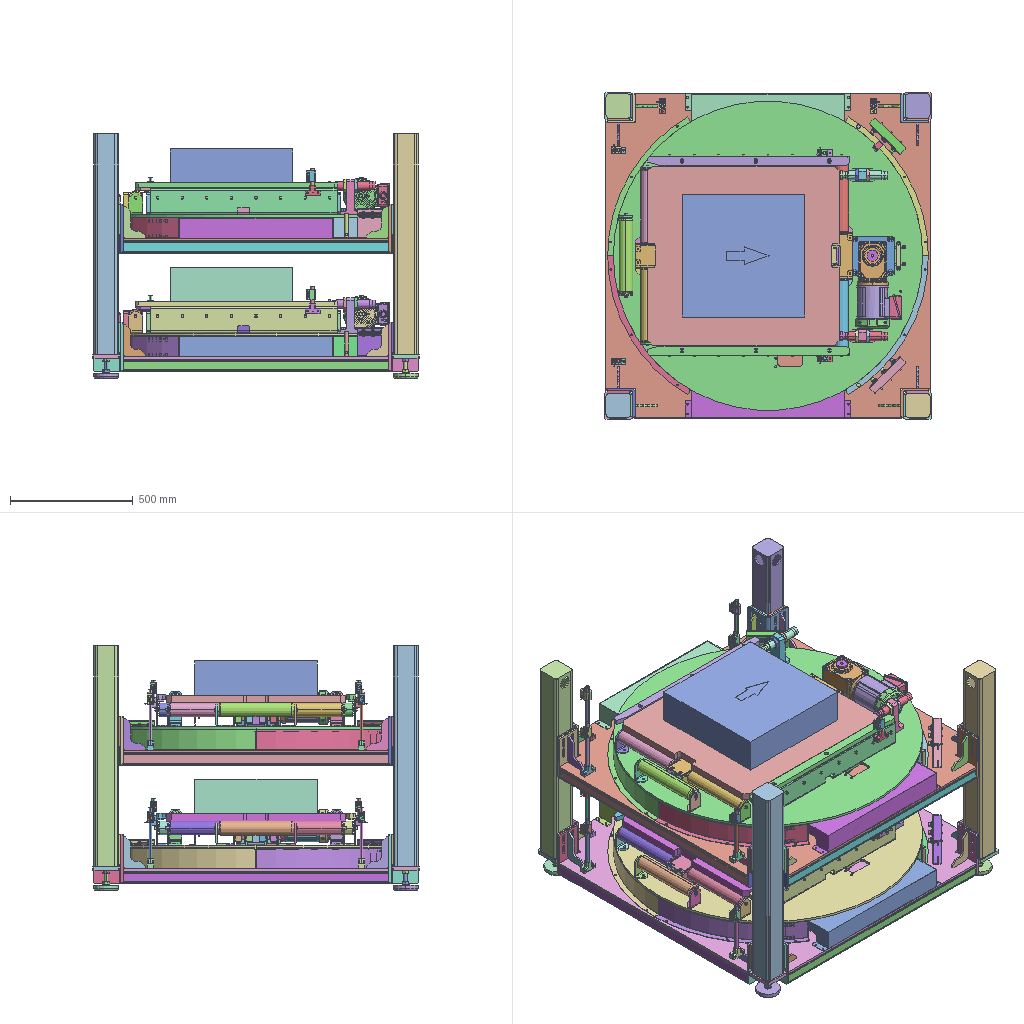Assembly | STEP file | 103 different items | 584 placed | box 1330 x 1330 x 995 mm
Parts list (item | name | quantity | parent item):
1 | diverter01.stp-1/DIVERTER.CONVEYOR.AS.stp-1/DIVERTER.AS.stp-1/BASE.FRAME.AS.stp-1/BASE.PLATE.1.stp-1-solid1 | x2 | in Solid 90-degree transfer
2 | diverter01.stp-1/DIVERTER.CONVEYOR.AS.stp-1/DIVERTER.AS.stp-1/BASE.FRAME.AS.stp-1/RIB.PLATE.1.stp-8-solid1 | x8 | in Solid 90-degree transfer
3 | diverter01.stp-1/DIVERTER.CONVEYOR.AS.stp-1/DIVERTER.AS.stp-1/BASE.FRAME.AS.stp-1/SQ.50.1.stp-4-solid1 | x8 | in Solid 90-degree transfer
4 | diverter01.stp-1/DIVERTER.CONVEYOR.AS.stp-1/DIVERTER.AS.stp-1/BASE.FRAME.AS.stp-1/SQ.50.3.stp-1-solid1 | x4 | in Solid 90-degree transfer
5 | diverter01.stp-1/DIVERTER.CONVEYOR.AS.stp-1/DIVERTER.AS.stp-1/CABLEVEYOR.AS.stp-1/CABLEVEYOR.BRACKET2.stp-1-solid1 | x2 | in Solid 90-degree transfer
6 | diverter01.stp-1/DIVERTER.CONVEYOR.AS.stp-1/DIVERTER.AS.stp-1/CABLEVEYOR.AS.stp-1/CABLEVEYOR.GUIDE.1.stp-1-solid1 | x2 | in Solid 90-degree transfer
7 | diverter01.stp-1/DIVERTER.CONVEYOR.AS.stp-1/DIVERTER.AS.stp-1/CABLEVEYOR.AS.stp-1/RV040CRA788639570230340-00503617.0690.stp-1/RV04CR.1.stp-1-solid1 | x2 | in Solid 90-degree transfer
8 | diverter01.stp-1/DIVERTER.CONVEYOR.AS.stp-1/DIVERTER.AS.stp-1/CONVEYOR.AS.stp-1/ROLLER.ASM.stp-1/HROJS57-313.stp-1/HROJS57-313_R.stp-1-solid1 (subassembly) | x2 | in Solid 90-degree transfer
9 | diverter01.stp-1/DIVERTER.CONVEYOR.AS.stp-1/DIVERTER.AS.stp-1/CONVEYOR.AS.stp-1/ROLLER.ASM.stp-1/HROJS57-313.stp-1/JNPN12_P.stp-1-solid1 (subassembly) | x2 | in Solid 90-degree transfer
10 | diverter01.stp-1/DIVERTER.CONVEYOR.AS.stp-1/DIVERTER.AS.stp-1/CONVEYOR.AS.stp-1/ROLLER.ASM.stp-1/MOR57-300-20.stp-12/MOR57-300-20BODY.stp-1-solid1 (subassembly) | x18 | in Solid 90-degree transfer
11 | diverter01.stp-1/DIVERTER.CONVEYOR.AS.stp-1/DIVERTER.AS.stp-1/CONVEYOR.AS.stp-1/ROLLER.ASM.stp-1/MOR57-300-20.stp-13/MOR57-300-10AC.stp-1-solid1 (subassembly) | x18 | in Solid 90-degree transfer
12 | diverter01.stp-1/DIVERTER.CONVEYOR.AS.stp-1/DIVERTER.AS.stp-1/CONVEYOR.AS.stp-1/ROLLER.ASM.stp-1/MOR57-300-20.stp-2/MOR57-300-20BODY.stp-1-solid1 (subassembly) | x18 | in Solid 90-degree transfer
13 | diverter01.stp-1/DIVERTER.CONVEYOR.AS.stp-1/DIVERTER.AS.stp-1/CONVEYOR.AS.stp-1/ROLLER.ASM.stp-1/MOR57-300-20.stp-5/MOR57-300-10AC.stp-1-solid1 (subassembly) | x18 | in Solid 90-degree transfer
14 | diverter01.stp-1/DIVERTER.CONVEYOR.AS.stp-1/DIVERTER.AS.stp-1/CONVEYOR.AS.stp-1/ROLLER.BRACKET.ASM.stp-1/ROLLER.BRACKET.3.stp-1-solid1 (subassembly) | x2 | in Solid 90-degree transfer
15 | diverter01.stp-1/DIVERTER.CONVEYOR.AS.stp-1/DIVERTER.AS.stp-1/CONVEYOR.AS.stp-1/ROLLER.BRACKET.ASM.stp-1/ROLLER.BRACKET.31.stp-2-solid1 (subassembly) | x2 | in Solid 90-degree transfer
16 | diverter01.stp-1/DIVERTER.CONVEYOR.AS.stp-1/DIVERTER.AS.stp-1/CONVEYOR.AS.stp-1/ROLLER.BRACKET.ASM.stp-1/ROLLER.BRACKET.33.stp-1-solid1 (subassembly) | x2 | in Solid 90-degree transfer
17 | diverter01.stp-1/DIVERTER.CONVEYOR.AS.stp-1/DIVERTER.AS.stp-1/CONVEYOR.AS.stp-1/ROLLER.BRACKET.ASM.stp-1/ROLLER.RBACKET.61.stp-1-solid1 (subassembly) | x2 | in Solid 90-degree transfer
18 | diverter01.stp-1/DIVERTER.CONVEYOR.AS.stp-1/DIVERTER.AS.stp-1/CONVEYOR.AS.stp-1/SIDE.GUIDE.2.stp-1-solid1 | x2 | in Solid 90-degree transfer
19 | diverter01.stp-1/DIVERTER.CONVEYOR.AS.stp-1/DIVERTER.AS.stp-1/END.STOPPER.AS.stp-1/ABSORBER.HOLDER.1.stp-2-solid1 | x4 | in Solid 90-degree transfer
20 | diverter01.stp-1/DIVERTER.CONVEYOR.AS.stp-1/DIVERTER.AS.stp-1/END.STOPPER.AS.stp-1/STOPPER.BRACKET.stp-1-solid1 | x2 | in Solid 90-degree transfer
21 | diverter01.stp-1/DIVERTER.CONVEYOR.AS.stp-1/DIVERTER.AS.stp-1/END.STOPPER.AS.stp-1/STOPPER.PAD.stp-1-solid1 | x2 | in Solid 90-degree transfer
22 | diverter01.stp-1/DIVERTER.CONVEYOR.AS.stp-1/DIVERTER.AS.stp-1/PALLET.ASM.1.stp-1/PALLET.UPPER.1.stp-1-solid1 (subassembly) | x2 | in Solid 90-degree transfer
23 | diverter01.stp-1/DIVERTER.CONVEYOR.AS.stp-1/DIVERTER.AS.stp-1/PX.SENSOR.ASM.stp-1/PR18-8DN.AS,.stp-1/PART1.stp-1-solid1 (subassembly) | x28 | in Solid 90-degree transfer
24 | diverter01.stp-1/DIVERTER.CONVEYOR.AS.stp-1/DIVERTER.AS.stp-1/PX.SENSOR.ASM.stp-1/PR18-8DN.AS,.stp-1/PR18-8DN.stp-1-solid1 (subassembly) | x2 | in Solid 90-degree transfer
25 | diverter01.stp-1/DIVERTER.CONVEYOR.AS.stp-1/DIVERTER.AS.stp-1/PX.SENSOR.ASM.stp-1/PR18-8DN.AS,.stp-3/PR18-8DN.stp-1-solid1 (subassembly) | x6 | in Solid 90-degree transfer
26 | diverter01.stp-1/DIVERTER.CONVEYOR.AS.stp-1/DIVERTER.AS.stp-1/PX.SENSOR.ASM.stp-1/PR18-8DN.AS,.stp-5/PR18-8DN.stp-1-solid1 (subassembly) | x2 | in Solid 90-degree transfer
27 | diverter01.stp-1/DIVERTER.CONVEYOR.AS.stp-1/DIVERTER.AS.stp-1/PX.SENSOR.ASM.stp-1/PR18-8DN.AS,.stp-6/PART2_1.stp-13-solid1 (subassembly) | x14 | in Solid 90-degree transfer
28 | diverter01.stp-1/DIVERTER.CONVEYOR.AS.stp-1/DIVERTER.AS.stp-1/PX.SENSOR.ASM.stp-1/SENSOR.BRACKET.11.stp-1-solid1 (subassembly) | x2 | in Solid 90-degree transfer
29 | diverter01.stp-1/DIVERTER.CONVEYOR.AS.stp-1/DIVERTER.AS.stp-1/PX.SENSOR.ASM.stp-1/SENSOR.BRACKET.2.stp-1-solid1 (subassembly) | x2 | in Solid 90-degree transfer
30 | diverter01.stp-1/DIVERTER.CONVEYOR.AS.stp-1/DIVERTER.AS.stp-1/SENSOR.ASM.stp-1/16-100.stp-1-solid1 (subassembly) | x4 | in Solid 90-degree transfer
31 | diverter01.stp-1/DIVERTER.CONVEYOR.AS.stp-1/DIVERTER.AS.stp-1/SENSOR.ASM.stp-1/16-250.stp-2-solid1 (subassembly) | x8 | in Solid 90-degree transfer
32 | diverter01.stp-1/DIVERTER.CONVEYOR.AS.stp-1/DIVERTER.AS.stp-1/SENSOR.ASM.stp-1/BJ7M-TDT.stp-1-solid8 (subassembly) | x2 | in Solid 90-degree transfer
33 | diverter01.stp-1/DIVERTER.CONVEYOR.AS.stp-1/DIVERTER.AS.stp-1/SENSOR.ASM.stp-1/BJ7M-TDT.stp-2-solid8 (subassembly) | x2 | in Solid 90-degree transfer
34 | diverter01.stp-1/DIVERTER.CONVEYOR.AS.stp-1/DIVERTER.AS.stp-1/SENSOR.ASM.stp-1/BJ7M-TDT.stp-3-solid2 (subassembly) | x2 | in Solid 90-degree transfer
35 | diverter01.stp-1/DIVERTER.CONVEYOR.AS.stp-1/DIVERTER.AS.stp-1/SENSOR.ASM.stp-1/BJ7M-TDT.stp-3-solid6 (subassembly) | x12 | in Solid 90-degree transfer
36 | diverter01.stp-1/DIVERTER.CONVEYOR.AS.stp-1/DIVERTER.AS.stp-1/SENSOR.ASM.stp-1/BJ7M-TDT.stp-3-solid7 (subassembly) | x6 | in Solid 90-degree transfer
37 | diverter01.stp-1/DIVERTER.CONVEYOR.AS.stp-1/DIVERTER.AS.stp-1/SENSOR.ASM.stp-1/BJ7M-TDT.stp-4-solid2 (subassembly) | x2 | in Solid 90-degree transfer
38 | diverter01.stp-1/DIVERTER.CONVEYOR.AS.stp-1/DIVERTER.AS.stp-1/SENSOR.ASM.stp-1/BJ7M-TDT.stp-5-solid3 (subassembly) | x12 | in Solid 90-degree transfer
39 | diverter01.stp-1/DIVERTER.CONVEYOR.AS.stp-1/DIVERTER.AS.stp-1/SENSOR.ASM.stp-1/BJ7M-TDT.stp-5-solid5 (subassembly) | x12 | in Solid 90-degree transfer
40 | diverter01.stp-1/DIVERTER.CONVEYOR.AS.stp-1/DIVERTER.AS.stp-1/SENSOR.ASM.stp-1/BJ7M-TDT.stp-6-solid7 (subassembly) | x6 | in Solid 90-degree transfer
41 | diverter01.stp-1/DIVERTER.CONVEYOR.AS.stp-1/DIVERTER.AS.stp-1/SENSOR.ASM.stp-1/PS16DH.SPM.stp-5-solid1 (subassembly) | x8 | in Solid 90-degree transfer
42 | diverter01.stp-1/DIVERTER.CONVEYOR.AS.stp-1/DIVERTER.AS.stp-1/SENSOR.ASM.stp-1/PS16RL.SPM.stp-2-solid1 (subassembly) | x6 | in Solid 90-degree transfer
43 | diverter01.stp-1/DIVERTER.CONVEYOR.AS.stp-1/DIVERTER.AS.stp-1/SENSOR.ASM.stp-1/PS16UL.SPM.stp-2-solid1 (subassembly) | x2 | in Solid 90-degree transfer
44 | diverter01.stp-1/DIVERTER.CONVEYOR.AS.stp-1/DIVERTER.AS.stp-1/SENSOR.ASM.stp-1/PS16UL.SPM.stp-3-solid1 (subassembly) | x4 | in Solid 90-degree transfer
45 | diverter01.stp-1/DIVERTER.CONVEYOR.AS.stp-1/DIVERTER.AS.stp-1/TURNING.AS.stp-1/HEX NUT - KS B 1012 - M8.stp-1-solid1 | x4 | in Solid 90-degree transfer
46 | diverter01.stp-1/DIVERTER.CONVEYOR.AS.stp-1/DIVERTER.AS.stp-1/TURNING.AS.stp-1/MOTOR.ASM.stp-1/F3S30N40-MM04TNNTN (subassembly) | x1 | in Solid 90-degree transfer
47 | diverter01.stp-1/DIVERTER.CONVEYOR.AS.stp-1/DIVERTER.AS.stp-1/TURNING.AS.stp-1/MOTOR.ASM.stp-1/GEAR.END.CAP.stp-2-solid1 (subassembly) | x4 | in Solid 90-degree transfer
48 | diverter01.stp-1/DIVERTER.CONVEYOR.AS.stp-1/DIVERTER.AS.stp-1/TURNING.AS.stp-1/MOTOR.ASM.stp-1/GEAR.SHAFT.stp-1-solid1 (subassembly) | x2 | in Solid 90-degree transfer
49 | diverter01.stp-1/DIVERTER.CONVEYOR.AS.stp-1/DIVERTER.AS.stp-1/TURNING.AS.stp-1/POST.AS.stp-1/POST.ASM.1.stp-13/M12.NUT.stp-1-solid1 (subassembly) | x22 | in Solid 90-degree transfer
50 | diverter01.stp-1/DIVERTER.CONVEYOR.AS.stp-1/DIVERTER.AS.stp-1/TURNING.AS.stp-1/POST.AS.stp-1/POST.ASM.1.stp-13/M12.WASHER.1.stp-1-solid1 (subassembly) | x32 | in Solid 90-degree transfer
51 | diverter01.stp-1/DIVERTER.CONVEYOR.AS.stp-1/DIVERTER.AS.stp-1/TURNING.AS.stp-1/POST.AS.stp-1/POST.ASM.1.stp-6/M12.NUT.stp-1-solid1 (subassembly) | x10 | in Solid 90-degree transfer
52 | - | x2 | in Solid 90-degree transfer
53 | diverter01.stp-1/DIVERTER.CONVEYOR.AS.stp-1/DIVERTER.AS.stp-1/TURNING.AS.stp-1/SPUR.6-20.stp-1-solid1 | x2 | in Solid 90-degree transfer
54 | diverter01.stp-1/DIVERTER.CONVEYOR.AS.stp-1/DIVERTER.AS.stp-2/BASE.FRAME.AS.stp-1/CORNER.BRACKET.1.stp-3-solid1 | x8 | in Solid 90-degree transfer
55 | diverter01.stp-1/DIVERTER.CONVEYOR.AS.stp-1/DIVERTER.AS.stp-2/BASE.FRAME.AS.stp-1/RIB.PLATE.1.stp-1-solid1 | x8 | in Solid 90-degree transfer
56 | diverter01.stp-1/DIVERTER.CONVEYOR.AS.stp-1/DIVERTER.AS.stp-2/BASE.FRAME.AS.stp-1/SQ.50.2.stp-1-solid1 | x2 | in Solid 90-degree transfer
57 | diverter01.stp-1/DIVERTER.CONVEYOR.AS.stp-1/DIVERTER.AS.stp-2/CABLEVEYOR.AS.stp-1/CABLEVEYOR.BRACKET.stp-1-solid1 | x2 | in Solid 90-degree transfer
58 | diverter01.stp-1/DIVERTER.CONVEYOR.AS.stp-1/DIVERTER.AS.stp-2/CABLEVEYOR.AS.stp-1/RV040CRA788639570230340-00503617.0690.stp-1/RV040CR-SU-40-50 | x2 | in Solid 90-degree transfer
59 | diverter01.stp-1/DIVERTER.CONVEYOR.AS.stp-1/DIVERTER.AS.stp-2/CABLEVEYOR.AS.stp-1/RV040CRA788639570230340-00503617.0690.stp-1/RV040CR_FB-78(2).stp-2-solid1 | x4 | in Solid 90-degree transfer
60 | diverter01.stp-1/DIVERTER.CONVEYOR.AS.stp-1/DIVERTER.AS.stp-2/CONVEYOR.AS.stp-1/ROLLER.ASM.stp-1/HROJS57-313.stp-1/HROJS57-313_PIN_S.stp-1-solid1 (subassembly) | x2 | in Solid 90-degree transfer
61 | diverter01.stp-1/DIVERTER.CONVEYOR.AS.stp-1/DIVERTER.AS.stp-2/CONVEYOR.AS.stp-1/ROLLER.BRACKET.ASM.stp-1/ROLLER.BRACKET.31.stp-1-solid1 (subassembly) | x2 | in Solid 90-degree transfer
62 | diverter01.stp-1/DIVERTER.CONVEYOR.AS.stp-1/DIVERTER.AS.stp-2/CONVEYOR.AS.stp-1/ROLLER.BRACKET.ASM.stp-1/ROLLER.BRACKET.33.stp-2-solid1 (subassembly) | x2 | in Solid 90-degree transfer
63 | diverter01.stp-1/DIVERTER.CONVEYOR.AS.stp-1/DIVERTER.AS.stp-2/CONVEYOR.AS.stp-1/ROLLER.BRACKET.ASM.stp-1/ROLLER.BRACKET.51.stp-1-solid1 (subassembly) | x2 | in Solid 90-degree transfer
64 | diverter01.stp-1/DIVERTER.CONVEYOR.AS.stp-1/DIVERTER.AS.stp-2/CONVEYOR.AS.stp-1/ROLLER.BRACKET.ASM.stp-1/ROLLER.BRACKET.52.stp-1-solid1 (subassembly) | x2 | in Solid 90-degree transfer
65 | diverter01.stp-1/DIVERTER.CONVEYOR.AS.stp-1/DIVERTER.AS.stp-2/CONVEYOR.AS.stp-1/ROLLER.BRACKET.ASM.stp-1/ROLLER.BRACKET.53.stp-1-solid1 (subassembly) | x2 | in Solid 90-degree transfer
66 | diverter01.stp-1/DIVERTER.CONVEYOR.AS.stp-1/DIVERTER.AS.stp-2/CONVEYOR.AS.stp-1/ROLLER.BRACKET.ASM.stp-1/ROLLER.RBACKET.61.stp-2-solid1 (subassembly) | x2 | in Solid 90-degree transfer
67 | diverter01.stp-1/DIVERTER.CONVEYOR.AS.stp-1/DIVERTER.AS.stp-2/CONVEYOR.AS.stp-1/SIDE.GUIDE.1.stp-1-solid1 | x2 | in Solid 90-degree transfer
68 | diverter01.stp-1/DIVERTER.CONVEYOR.AS.stp-1/DIVERTER.AS.stp-2/CONVEYOR.AS.stp-1/UPPER.COVER.1.stp-1-solid1 | x2 | in Solid 90-degree transfer
69 | diverter01.stp-1/DIVERTER.CONVEYOR.AS.stp-1/DIVERTER.AS.stp-2/END.STOPPER.AS.stp-1/C-AD3650.stp-1/C-AD3650-ROD_R.stp-1-solid1 | x4 | in Solid 90-degree transfer
70 | diverter01.stp-1/DIVERTER.CONVEYOR.AS.stp-1/DIVERTER.AS.stp-2/END.STOPPER.AS.stp-1/C-AD3650.stp-1/C-AD3650_B.stp-1-solid1 | x4 | in Solid 90-degree transfer
71 | diverter01.stp-1/DIVERTER.CONVEYOR.AS.stp-1/DIVERTER.AS.stp-2/END.STOPPER.AS.stp-1/C-AD3650.stp-2/C-AD3650-NUT_N.stp-2-solid1 | x8 | in Solid 90-degree transfer
72 | diverter01.stp-1/DIVERTER.CONVEYOR.AS.stp-1/DIVERTER.AS.stp-2/OUTER.COVER.AS.stp-1/OUTER.COVER.1.stp-1-solid1 | x8 | in Solid 90-degree transfer
73 | diverter01.stp-1/DIVERTER.CONVEYOR.AS.stp-1/DIVERTER.AS.stp-2/OUTER.COVER.AS.stp-1/OUTER.COVER.2.stp-1-solid1 | x2 | in Solid 90-degree transfer
74 | diverter01.stp-1/DIVERTER.CONVEYOR.AS.stp-1/DIVERTER.AS.stp-2/OUTER.COVER.AS.stp-1/OUTER.COVER.2.stp-2-solid1 | x2 | in Solid 90-degree transfer
75 | diverter01.stp-1/DIVERTER.CONVEYOR.AS.stp-1/DIVERTER.AS.stp-2/PALLET.ASM.1.stp-1/PALLET.1.stp-1-solid1 (subassembly) | x2 | in Solid 90-degree transfer
76 | diverter01.stp-1/DIVERTER.CONVEYOR.AS.stp-1/DIVERTER.AS.stp-2/PX.SENSOR.ASM.stp-1/PR18-8DN.AS,.stp-7/PR18-8DN.stp-1-solid1 (subassembly) | x4 | in Solid 90-degree transfer
77 | diverter01.stp-1/DIVERTER.CONVEYOR.AS.stp-1/DIVERTER.AS.stp-2/PX.SENSOR.ASM.stp-1/SENSOR.BRACKET.2.stp-2-solid1 (subassembly) | x2 | in Solid 90-degree transfer
78 | diverter01.stp-1/DIVERTER.CONVEYOR.AS.stp-1/DIVERTER.AS.stp-2/SENSOR.ASM.stp-1/BJ7M-TDT.stp-1-solid2 (subassembly) | x4 | in Solid 90-degree transfer
79 | diverter01.stp-1/DIVERTER.CONVEYOR.AS.stp-1/DIVERTER.AS.stp-2/SENSOR.ASM.stp-1/BJ7M-TDT.stp-3-solid8 (subassembly) | x2 | in Solid 90-degree transfer
80 | diverter01.stp-1/DIVERTER.CONVEYOR.AS.stp-1/DIVERTER.AS.stp-2/SENSOR.ASM.stp-1/BJ7M-TDT.stp-4-solid8 (subassembly) | x2 | in Solid 90-degree transfer
81 | diverter01.stp-1/DIVERTER.CONVEYOR.AS.stp-1/DIVERTER.AS.stp-2/SENSOR.ASM.stp-1/BJ7M-TDT.stp-5-solid8 (subassembly) | x2 | in Solid 90-degree transfer
82 | diverter01.stp-1/DIVERTER.CONVEYOR.AS.stp-1/DIVERTER.AS.stp-2/SENSOR.ASM.stp-1/BJ7M-TDT.stp-6-solid1 (subassembly) | x12 | in Solid 90-degree transfer
83 | diverter01.stp-1/DIVERTER.CONVEYOR.AS.stp-1/DIVERTER.AS.stp-2/SENSOR.ASM.stp-1/BJ7M-TDT.stp-6-solid2 (subassembly) | x4 | in Solid 90-degree transfer
84 | diverter01.stp-1/DIVERTER.CONVEYOR.AS.stp-1/DIVERTER.AS.stp-2/SENSOR.ASM.stp-1/BJ7M-TDT.stp-6-solid4 (subassembly) | x12 | in Solid 90-degree transfer
85 | diverter01.stp-1/DIVERTER.CONVEYOR.AS.stp-1/DIVERTER.AS.stp-2/SENSOR.ASM.stp-1/BJ7M-TDT.stp-6-solid8 (subassembly) | x2 | in Solid 90-degree transfer
86 | diverter01.stp-1/DIVERTER.CONVEYOR.AS.stp-1/DIVERTER.AS.stp-2/SENSOR.ASM.stp-1/PS16DH.SPM.stp-4-solid1 (subassembly) | x4 | in Solid 90-degree transfer
87 | diverter01.stp-1/DIVERTER.CONVEYOR.AS.stp-1/DIVERTER.AS.stp-2/STOPPER.BAR.stp-2-solid1 | x4 | in Solid 90-degree transfer
88 | diverter01.stp-1/DIVERTER.CONVEYOR.AS.stp-1/DIVERTER.AS.stp-2/TURN.TABLE.1.stp-1-solid1 | x2 | in Solid 90-degree transfer
89 | diverter01.stp-1/DIVERTER.CONVEYOR.AS.stp-1/DIVERTER.AS.stp-2/TURNING.AS.stp-1/BOLTS.AS.stp-1/M16.W.P.30L.stp-5-solid1 | x24 | in Solid 90-degree transfer
90 | diverter01.stp-1/DIVERTER.CONVEYOR.AS.stp-1/DIVERTER.AS.stp-2/TURNING.AS.stp-1/HEX-HEAD BOLT - KS B 1002 - A M8X40.stp-1-solid1 | x4 | in Solid 90-degree transfer
91 | diverter01.stp-1/DIVERTER.CONVEYOR.AS.stp-1/DIVERTER.AS.stp-2/TURNING.AS.stp-1/MOTOR.ASM.stp-1/F3S30N40-MM04TNNTN (subassembly) | x1 | in Solid 90-degree transfer
92 | diverter01.stp-1/DIVERTER.CONVEYOR.AS.stp-1/DIVERTER.AS.stp-2/TURNING.AS.stp-1/MOTOR.MOUNT.1.stp-1-solid1 | x2 | in Solid 90-degree transfer
93 | diverter01.stp-1/DIVERTER.CONVEYOR.AS.stp-1/DIVERTER.AS.stp-2/TURNING.AS.stp-1/POST.AS.stp-1/POST.ASM.1.stp-3/POST.BOLT.1.stp-1-solid1 (subassembly) | x32 | in Solid 90-degree transfer
94 | - | x2 | in Solid 90-degree transfer
95 | - | x2 | in Solid 90-degree transfer
96 | diverter01.stp-1/DIVERTER.CONVEYOR.AS.stp-1/DIVERTER.AS.stp-2/TURNING.AS.stp-1/TENSION.BLOCK.stp-1-solid1 | x2 | in Solid 90-degree transfer
97 | diverter01.stp-1/DIVERTER.CONVEYOR.AS.stp-1/DIVERTER.AS.stp-2/TURNING.STOPPER.BLOCK.stp-1-solid1 | x2 | in Solid 90-degree transfer
98 | diverter01.stp-1/DIVERTER.CONVEYOR.AS.stp-1/POST.FRAME.AS.stp-1/POST.ASM.stp-1/FJKF16-120.stp-1/FJKB16-98NUT.stp-1-solid1 (subassembly) | x4 | in Solid 90-degree transfer
99 | diverter01.stp-1/DIVERTER.CONVEYOR.AS.stp-1/POST.FRAME.AS.stp-1/POST.ASM.stp-1/LEVEL.PAD.1.stp-1-solid1 (subassembly) | x4 | in Solid 90-degree transfer
100 | diverter01.stp-1/DIVERTER.CONVEYOR.AS.stp-1/POST.FRAME.AS.stp-1/POST.ASM.stp-2/ATTACH.PLATE.1.stp-1-solid1 (subassembly) | x16 | in Solid 90-degree transfer
101 | diverter01.stp-1/DIVERTER.CONVEYOR.AS.stp-1/POST.FRAME.AS.stp-1/POST.ASM.stp-2/POST.SQ.PIPE.stp-1-solid1 (subassembly) | x4 | in Solid 90-degree transfer
102 | diverter01.stp-1/DIVERTER.CONVEYOR.AS.stp-1/POST.FRAME.AS.stp-1/POST.ASM.stp-3/FJKF16-120.stp-1/FJKF16-120BOLT.stp-1-solid1 (subassembly) | x4 | in Solid 90-degree transfer
103 | diverter01.stp-1/DIVERTER.CONVEYOR.AS.stp-1/POST.FRAME.AS.stp-1/POST.ASM.stp-3/SEPLC100-20.stp-1-solid1 (subassembly) | x4 | in Solid 90-degree transfer